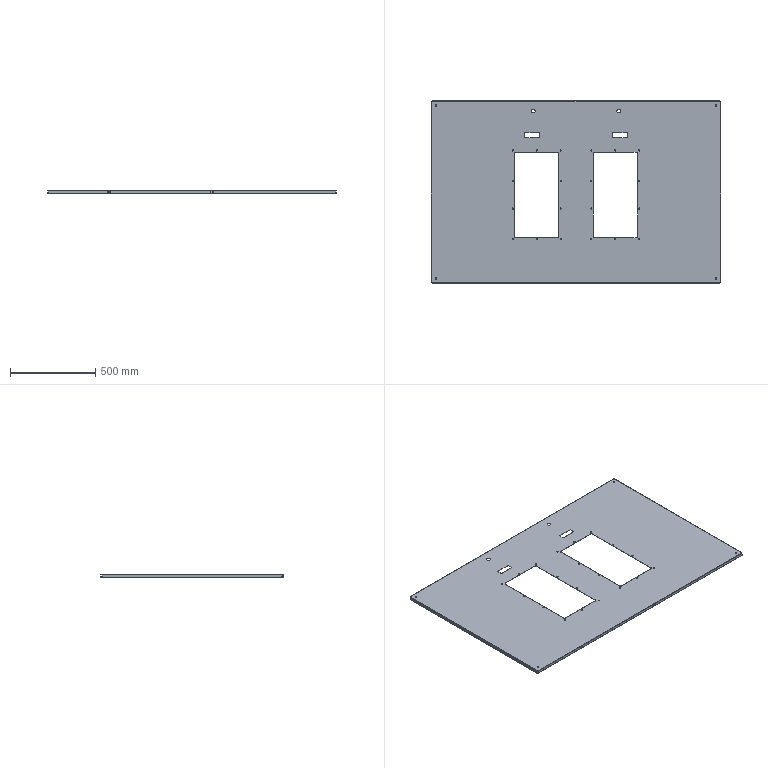Part | SolidWorks | features BaseBody 1 | 1 solid | 134 faces | box 1696 x 1066 x 18 mm | volume 2491108 mm3 | cylinder 80 | plane 54 | commonest cylinder face diameters 7 x40 9 x8 22 x8 1.473 x6 4.473 x6 6.5 x4